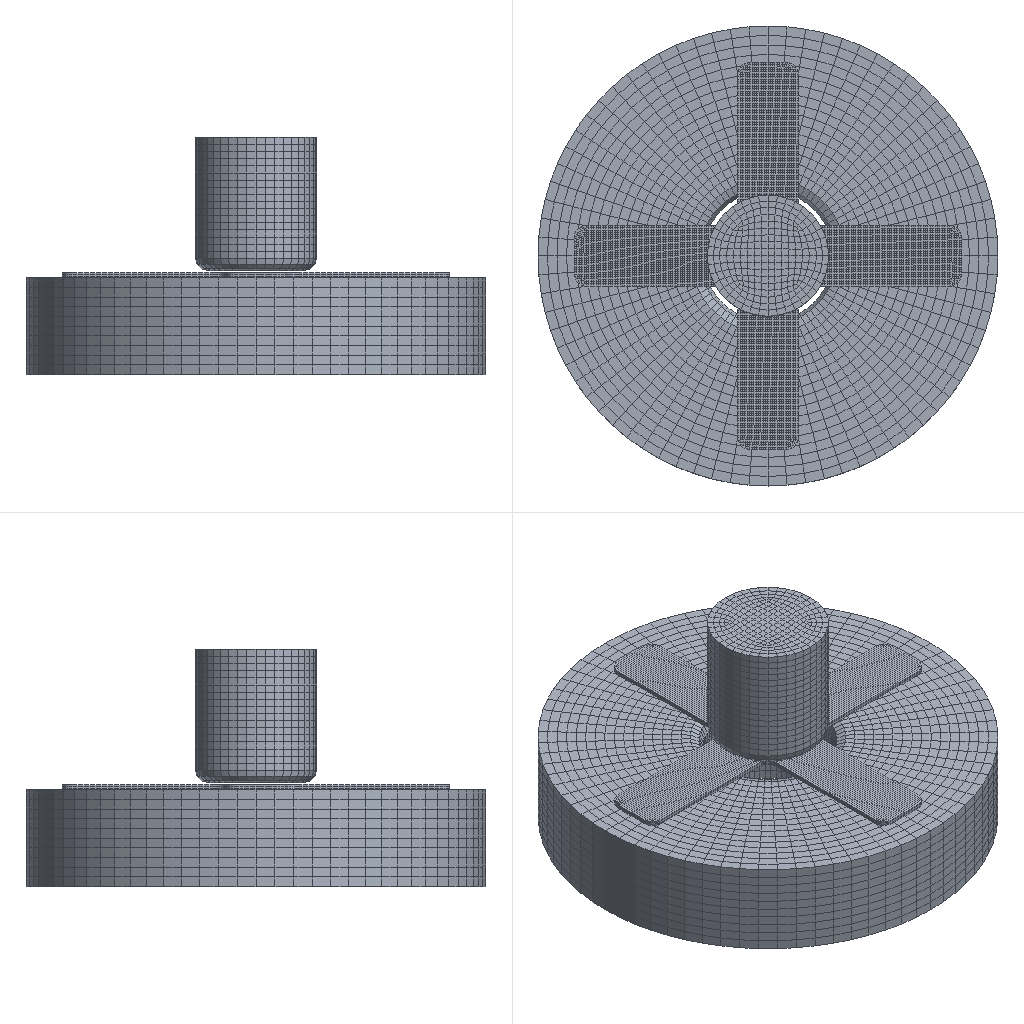Simulation study | abaqus
Set-up summary:
category,name,step,type,value,unit,region
solver,abaqus
solver,version,,,Abaqus/Explicit 2020
units,not stated in the deck,,not stated
analysis,deck,,transient,transient
load_step,Step-1,Step-1,transient
load_step,requested,,,1
mesh,nodes,,,52959
mesh,elements,,,41340
element_type,C3D8R,,solid,41340
load,load commands in deck,,count,1
bc,support commands in deck,,count,8
material,AZ31,,in results
check,setup vs results,,match,"per instance, exact: element labels, types and connectivity; labels of the nodes the elements use; coordinates not compared"
Abaqus input file, long lists of numbers shortened:
*Heading
** Job name: [REDACTED] Model name: Model-2-xiantan
** Generated by: Abaqus/CAE 2020
*Preprint, echo=NO, model=NO, history=NO, contact=NO
**
** PARTS
**
*Part, name=die
*Node
      1,           0.,          32.,           0.
      2,           0.,          32.,          40.
** (15806 more lines like these left out)
*Element, type=C3D8R
   1,  162, 1549, 5369, 1009,    1,   25,  685,   78
   2, 1549, 1550, 5370, 5369,   25,   26,  686,  685
** (13678 more lines like these left out)
*Nset, nset=_PickedSet6, internal, generate
     1,  15808,      1
*Elset, elset=_PickedSet6, internal, generate
     1,  13680,      1
** Section: Section-1
*Solid Section, elset=_PickedSet6, material=az31
,
*End Part
**
*Part, name=punch
*Node
      1,           0.,          20.,          55.
      2,           0.,           0.,          55.
** (5577 more lines like these left out)
*Element, type=C3D8R
  1,  508,  509, 2634, 2470,   23,   24,  373,  372
  2,  509,  510, 2635, 2634,   24,   25,  374,  373
** (4918 more lines like these left out)
*Nset, nset=_PickedSet5, internal, generate
    1,  5579,     1
*Elset, elset=_PickedSet5, internal, generate
    1,  4920,     1
** Section: Section-1
*Solid Section, elset=_PickedSet5, material=az31
,
*End Part
**
*Part, name=work
*Node
      1,   2.55,  -17.461,           0.
      2,   3.446,  -2.526,           0.
** (31570 more lines like these left out)
*Element, type=C3D8R
    1,   930,   942,    43,    42,  8823,  8835,  7936,  7935
    2,   942,   943,    44,    43,  8835,  8836,  7937,  7936
** (22738 more lines like these left out)
*Nset, nset=_PickedSet2, internal, generate
     1,  31572,      1
*Elset, elset=_PickedSet2, internal, generate
     1,  22740,      1
** Section: Section-1
*Solid Section, elset=_PickedSet2, material=az31
,
*End Part
**
**
** ASSEMBLY
**
*Assembly, name=Assembly
**
*Instance, name=die-1, part=die
*End Instance
**
*Instance, name=work-1, part=work
          0.,           0.,          40.
*End Instance
**
*Instance, name=punch-1, part=punch
          0.,           0.,          98.
          0.,           0.,          98.,           1.,           0.,          98.,         180.
*End Instance
**
*Node
      1,           0.,           0.,          98.
*Node
      2,           0., 5.81707246e-15,           0.
*Nset, nset=Set-die
 2,
*Nset, nset=Set-punch
 1,
*Nset, nset=_PickedSet20, internal, instance=punch-1, generate
    1,  5579,     1
*Elset, elset=_PickedSet20, internal, instance=punch-1, generate
    1,  4920,     1
*Nset, nset=_PickedSet27, internal, instance=die-1, generate
     1,  15808,      1
*Elset, elset=_PickedSet27, internal, instance=die-1, generate
     1,  13680,      1
*Elset, elset=__PickedSurf30_S6, internal, instance=punch-1
 3241, 3242, 3244, 3245, 3256, 3258, 3272, 3275, 3283, 3284, 3286, 3287, 3298, 3300, 3314, 3317
 3325, 3326, 3328, 3329, 3340, 3342, 3356, 3359, 3367, 3368, 3370, 3371, 3382, 3384, 3398, 3401
** (18 more lines like these left out)
*Elset, elset=__PickedSurf30_S5, internal, instance=punch-1
 3247, 3249, 3251, 3252, 3254, 3263, 3264, 3267, 3268, 3271, 3289, 3291, 3293, 3294, 3296, 3305
 3306, 3309, 3310, 3313, 3331, 3333, 3335, 3336, 3338, 3347, 3348, 3351, 3352, 3355, 3373, 3375
** (23 more lines like these left out)
*Elset, elset=__PickedSurf30_S4, internal, instance=punch-1
 2034, 2043, 2052, 2061, 2070, 2079, 2088, 2097, 2106, 2115, 2844, 2853, 2862, 2871, 2880, 2889
 2898, 2907, 2916, 2925, 3024, 3033, 3042, 3051, 3060, 3069, 3078, 3087, 3096, 3105, 3114, 3123
** (6 more lines like these left out)
*Elset, elset=__PickedSurf30_S2, internal, instance=punch-1
    1,    2,    3,    4,    5,    6,    7,    8,    9,   10,   91,   92,   93,   94,   95,   96
   97,   98,   99,  100,  101,  102,  103,  104,  105,  106,  107,  108,  109,  110,  111,  112
** (4 more lines like these left out)
*Elset, elset=__PickedSurf30_S3, internal, instance=punch-1
 2116, 2117, 2118, 2119, 2120, 2161, 2162, 2163, 2164, 2165, 2206, 2207, 2208, 2209, 2210, 2251
 2252, 2253, 2254, 2255, 2296, 2297, 2298, 2299, 2300, 2341, 2342, 2343, 2344, 2345, 2386, 2387
** (1 more lines like these left out)
*Surface, type=ELEMENT, name=_PickedSurf30, internal
__PickedSurf30_S6, S6
__PickedSurf30_S5, S5
__PickedSurf30_S4, S4
__PickedSurf30_S2, S2
__PickedSurf30_S3, S3
*Elset, elset=__PickedSurf31_S2, internal, instance=work-1, generate
 15161,  22740,      1
*Surface, type=ELEMENT, name=_PickedSurf31, internal
__PickedSurf31_S2, S2
*Elset, elset=__PickedSurf32_S6, internal, instance=die-1
  3041,  3051,  3061,  3071,  3081,  3091,  3101,  3111,  3121,  3131,  3141,  3151,  3161,  3171,  3181,  3191
  3201,  3211,  3221,  3231,  3241,  3251,  3261,  3271,  3281,  3291,  3301,  3311,  3321,  3331,  3341,  3351
** (55 more lines like these left out)
*Elset, elset=__PickedSurf32_S4, internal, instance=die-1
    10,    20,    30,    40,    50,    60,    70,    80,    90,   100,   110,   120,   130,   140,   150,   160
   170,   180,   190,   200,   210,   220,   230,   240,   250,   260,   270,   280,   290,   300,   310,   320
** (51 more lines like these left out)
*Elset, elset=__PickedSurf32_S2, internal, instance=die-1, generate
 9121,  9424,     1
*Surface, type=ELEMENT, name=_PickedSurf32, internal
__PickedSurf32_S6, S6
__PickedSurf32_S4, S4
__PickedSurf32_S2, S2
*Elset, elset=__PickedSurf33_S1, internal, instance=work-1, generate
    1,  7580,     1
*Surface, type=ELEMENT, name=_PickedSurf33, internal
__PickedSurf33_S1, S1
** Constraint: Constraint-1
*Rigid Body, ref node=Set-punch, elset=_PickedSet20
** Constraint: Constraint-2
*Rigid Body, ref node=Set-die, elset=_PickedSet27
*End Assembly
**
** MATERIALS
**
*Material, name=az31
*Density
 1.78e-09,
*Elastic
45000., 0.35
**
** INTERACTION PROPERTIES
**
*Surface Interaction, name=IntProp-1
*Friction
 0.15,
*Surface Behavior, pressure-overclosure=HARD
**
** BOUNDARY CONDITIONS
**
** Name: BC-1 Type: 对称/反对称/完全固定
*Boundary
Set-die, ENCASTRE
** Name: BC-2 Type: 速度/角速度
*Boundary, type=VELOCITY
Set-punch, 1, 1
Set-punch, 2, 2
Set-punch, 3, 3
Set-punch, 4, 4
Set-punch, 5, 5
Set-punch, 6, 6
** ----------------------------------------------------------------
**
** STEP: Step-1
**
*Step, name=Step-1, nlgeom=YES
*Dynamic, Explicit
, 0.05
*Bulk Viscosity
0.06, 1.2
** Mass Scaling: Semi-Automatic
**               Whole Model
*Fixed Mass Scaling, factor=200.
**
** BOUNDARY CONDITIONS
**
** Name: BC-2 Type: 速度/角速度
*Boundary, type=VELOCITY
Set-punch, 3, 3, -600.
**
** INTERACTIONS
**
** Interaction: Int-1
*Contact Pair, interaction=IntProp-1, mechanical constraint=PENALTY, cpset=Int-1
_PickedSurf30, _PickedSurf31
** Interaction: Int-2
*Contact Pair, interaction=IntProp-1, mechanical constraint=PENALTY, cpset=Int-2
_PickedSurf32, _PickedSurf33
**
** OUTPUT REQUESTS
**
*Restart, write, number interval=1, time marks=NO
**
** FIELD OUTPUT: F-Output-1
**
*Output, field, number interval=100
*Node Output
RF, U
*Element Output, directions=YES
LE, PE, PEEQ, S
**
** HISTORY OUTPUT: H-Output-1
**
*Output, history, variable=PRESELECT
*End Step
Results summary:
result,step,Step-1,completed,increments=45597 time=0.05/0.05
result,analysis,,,transient
result,last_loadstep,,,1
result,primary field,,,U
result,reaction total,,FX,3115.631,model units
result,reaction total,,FY,-5402.796,model units
result,reaction total,,FZ,2884.322,model units